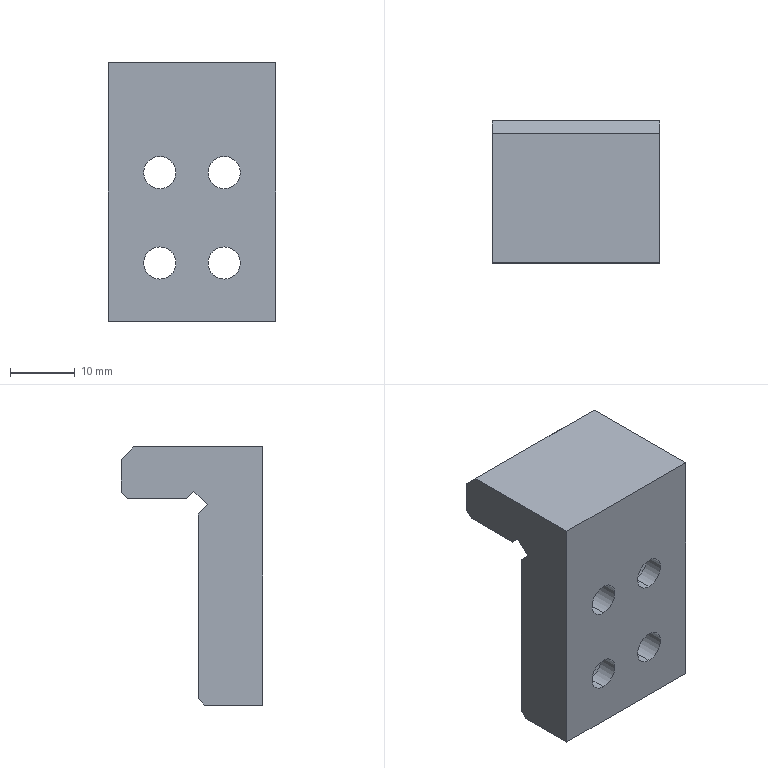Part | SolidWorks | features Chamfer 2, Cut 2, ICE 2, Extrusion 1, HoleWzd 1 | 1 solid | 28 faces | box 26 x 22 x 40 mm | volume 10641 mm3 | plane 16 | cylinder 12 | commonest cylinder face diameters 5 x8 12 x4
STEP:
#1=CARTESIAN_POINT('',(5.,3.,-3.));
#2=VERTEX_POINT('',#1);
#3=CARTESIAN_POINT('',(5.,3.,9.));
#4=VERTEX_POINT('',#3);
#5=CARTESIAN_POINT('',(5.,3.,3.));
#6=DIRECTION('',(0.,1.,0.));
#7=DIRECTION('',(0.,0.,1.));
#8=AXIS2_PLACEMENT_3D('',#5,#6,#7);
#9=CIRCLE('',#8,6.);
#10=EDGE_CURVE('',#2,#4,#9,.T.);
#11=ORIENTED_EDGE('',*,*,#10,.F.);
#12=CARTESIAN_POINT('',(5.,10.,-3.));
#13=VERTEX_POINT('',#12);
#14=CARTESIAN_POINT('',(5.,3.,-3.));
#15=DIRECTION('',(0.,1.,0.));
#16=VECTOR('',#15,1000.);
#17=LINE('',#14,#16);
#18=EDGE_CURVE('',#2,#13,#17,.T.);
#19=ORIENTED_EDGE('',*,*,#18,.T.);
#20=CARTESIAN_POINT('',(5.,10.,9.));
#21=VERTEX_POINT('',#20);
#22=CARTESIAN_POINT('',(5.,10.,3.));
#23=DIRECTION('',(0.,1.,0.));
#24=DIRECTION('',(0.,0.,1.));
#25=AXIS2_PLACEMENT_3D('',#22,#23,#24);
#26=CIRCLE('',#25,6.);
#27=EDGE_CURVE('',#13,#21,#26,.T.);
#28=ORIENTED_EDGE('',*,*,#27,.T.);
#29=CARTESIAN_POINT('',(5.,3.,9.));
#30=DIRECTION('',(0.,1.,0.));
#31=VECTOR('',#30,1000.);
#32=LINE('',#29,#31);
#33=EDGE_CURVE('',#4,#21,#32,.T.);
#34=ORIENTED_EDGE('',*,*,#33,.F.);
#35=EDGE_LOOP('',(#11,#19,#28,#34));
#36=FACE_OUTER_BOUND('',#35,.T.);
#37=CARTESIAN_POINT('',(5.,3.,3.));
#38=DIRECTION('',(0.,1.,0.));
#39=DIRECTION('',(0.,0.,1.));
#40=AXIS2_PLACEMENT_3D('',#37,#38,#39);
#41=CYLINDRICAL_SURFACE('',#40,6.);
#42=ADVANCED_FACE('',(#36),#41,.F.);
#43=CARTESIAN_POINT('',(-5.,3.,-17.));
#44=VERTEX_POINT('',#43);
#45=CARTESIAN_POINT('',(-5.,3.,-5.));
#46=VERTEX_POINT('',#45);
#47=CARTESIAN_POINT('',(-5.,3.,-11.));
#48=DIRECTION('',(0.,1.,0.));
#49=DIRECTION('',(0.,0.,1.));
#50=AXIS2_PLACEMENT_3D('',#47,#48,#49);
#51=CIRCLE('',#50,6.);
#52=EDGE_CURVE('',#44,#46,#51,.T.);
#53=ORIENTED_EDGE('',*,*,#52,.F.);
#54=CARTESIAN_POINT('',(-5.,10.,-17.));
#55=VERTEX_POINT('',#54);
#56=CARTESIAN_POINT('',(-5.,3.,-17.));
#57=DIRECTION('',(0.,1.,0.));
#58=VECTOR('',#57,1000.);
#59=LINE('',#56,#58);
#60=EDGE_CURVE('',#44,#55,#59,.T.);
#61=ORIENTED_EDGE('',*,*,#60,.T.);
#62=CARTESIAN_POINT('',(-5.,10.,-5.));
#63=VERTEX_POINT('',#62);
#64=CARTESIAN_POINT('',(-5.,10.,-11.));
#65=DIRECTION('',(0.,1.,0.));
#66=DIRECTION('',(0.,0.,1.));
#67=AXIS2_PLACEMENT_3D('',#64,#65,#66);
#68=CIRCLE('',#67,6.);
#69=EDGE_CURVE('',#55,#63,#68,.T.);
#70=ORIENTED_EDGE('',*,*,#69,.T.);
#71=CARTESIAN_POINT('',(-5.,3.,-5.));
#72=DIRECTION('',(0.,1.,0.));
#73=VECTOR('',#72,1000.);
#74=LINE('',#71,#73);
#75=EDGE_CURVE('',#46,#63,#74,.T.);
#76=ORIENTED_EDGE('',*,*,#75,.F.);
#77=EDGE_LOOP('',(#53,#61,#70,#76));
#78=FACE_OUTER_BOUND('',#77,.T.);
#79=CARTESIAN_POINT('',(-5.,3.,-11.));
#80=DIRECTION('',(0.,1.,0.));
#81=DIRECTION('',(0.,0.,1.));
#82=AXIS2_PLACEMENT_3D('',#79,#80,#81);
#83=CYLINDRICAL_SURFACE('',#82,6.);
#84=ADVANCED_FACE('',(#78),#83,.F.);
#85=CARTESIAN_POINT('',(5.,0.,-13.5));
#86=VERTEX_POINT('',#85);
#87=CARTESIAN_POINT('',(5.,0.,-8.5));
#88=VERTEX_POINT('',#87);
#89=CARTESIAN_POINT('',(5.,0.,-11.));
#90=DIRECTION('',(0.,1.,0.));
#91=DIRECTION('',(0.,0.,1.));
#92=AXIS2_PLACEMENT_3D('',#89,#90,#91);
#93=CIRCLE('',#92,2.5);
#94=EDGE_CURVE('',#86,#88,#93,.T.);
#95=ORIENTED_EDGE('',*,*,#94,.F.);
#96=CARTESIAN_POINT('',(5.,10.,-13.5));
#97=VERTEX_POINT('',#96);
#98=CARTESIAN_POINT('',(5.,0.,-13.5));
#99=DIRECTION('',(0.,1.,0.));
#100=VECTOR('',#99,1000.);
#101=LINE('',#98,#100);
#102=EDGE_CURVE('',#86,#97,#101,.T.);
#103=ORIENTED_EDGE('',*,*,#102,.T.);
#104=CARTESIAN_POINT('',(5.,10.,-8.5));
#105=VERTEX_POINT('',#104);
#106=CARTESIAN_POINT('',(5.,10.,-11.));
#107=DIRECTION('',(0.,1.,0.));
#108=DIRECTION('',(0.,0.,1.));
#109=AXIS2_PLACEMENT_3D('',#106,#107,#108);
#110=CIRCLE('',#109,2.5);
#111=EDGE_CURVE('',#97,#105,#110,.T.);
#112=ORIENTED_EDGE('',*,*,#111,.T.);
#113=CARTESIAN_POINT('',(5.,0.,-8.5));
#114=DIRECTION('',(0.,1.,0.));
#115=VECTOR('',#114,1000.);
#116=LINE('',#113,#115);
#117=EDGE_CURVE('',#88,#105,#116,.T.);
#118=ORIENTED_EDGE('',*,*,#117,.F.);
#119=EDGE_LOOP('',(#95,#103,#112,#118));
#120=FACE_OUTER_BOUND('',#119,.T.);
#121=CARTESIAN_POINT('',(5.,0.,-11.));
#122=DIRECTION('',(0.,1.,0.));
#123=DIRECTION('',(0.,0.,1.));
#124=AXIS2_PLACEMENT_3D('',#121,#122,#123);
#125=CYLINDRICAL_SURFACE('',#124,2.5);
#126=ADVANCED_FACE('',(#120),#125,.F.);
#127=CARTESIAN_POINT('',(-5.,0.,0.5));
#128=VERTEX_POINT('',#127);
#129=CARTESIAN_POINT('',(-5.,0.,5.5));
#130=VERTEX_POINT('',#129);
#131=CARTESIAN_POINT('',(-5.,0.,3.));
#132=DIRECTION('',(0.,1.,0.));
#133=DIRECTION('',(0.,0.,1.));
#134=AXIS2_PLACEMENT_3D('',#131,#132,#133);
#135=CIRCLE('',#134,2.5);
#136=EDGE_CURVE('',#128,#130,#135,.T.);
#137=ORIENTED_EDGE('',*,*,#136,.F.);
#138=CARTESIAN_POINT('',(-5.,10.,0.5));
#139=VERTEX_POINT('',#138);
#140=CARTESIAN_POINT('',(-5.,0.,0.5));
#141=DIRECTION('',(0.,1.,0.));
#142=VECTOR('',#141,1000.);
#143=LINE('',#140,#142);
#144=EDGE_CURVE('',#128,#139,#143,.T.);
#145=ORIENTED_EDGE('',*,*,#144,.T.);
#146=CARTESIAN_POINT('',(-5.,10.,5.5));
#147=VERTEX_POINT('',#146);
#148=CARTESIAN_POINT('',(-5.,10.,3.));
#149=DIRECTION('',(0.,1.,0.));
#150=DIRECTION('',(0.,0.,1.));
#151=AXIS2_PLACEMENT_3D('',#148,#149,#150);
#152=CIRCLE('',#151,2.5);
#153=EDGE_CURVE('',#139,#147,#152,.T.);
#154=ORIENTED_EDGE('',*,*,#153,.T.);
#155=CARTESIAN_POINT('',(-5.,0.,5.5));
#156=DIRECTION('',(0.,1.,0.));
#157=VECTOR('',#156,1000.);
#158=LINE('',#155,#157);
#159=EDGE_CURVE('',#130,#147,#158,.T.);
#160=ORIENTED_EDGE('',*,*,#159,.F.);
#161=EDGE_LOOP('',(#137,#145,#154,#160));
#162=FACE_OUTER_BOUND('',#161,.T.);
#163=CARTESIAN_POINT('',(-5.,0.,3.));
#164=DIRECTION('',(0.,1.,0.));
#165=DIRECTION('',(0.,0.,1.));
#166=AXIS2_PLACEMENT_3D('',#163,#164,#165);
#167=CYLINDRICAL_SURFACE('',#166,2.5);
#168=ADVANCED_FACE('',(#162),#167,.F.);
#169=CARTESIAN_POINT('',(-5.,0.,-13.5));
#170=VERTEX_POINT('',#169);
#171=CARTESIAN_POINT('',(-5.,0.,-8.5));
#172=VERTEX_POINT('',#171);
#173=CARTESIAN_POINT('',(-5.,0.,-11.));
#174=DIRECTION('',(0.,1.,0.));
#175=DIRECTION('',(0.,0.,1.));
#176=AXIS2_PLACEMENT_3D('',#173,#174,#175);
#177=CIRCLE('',#176,2.5);
#178=EDGE_CURVE('',#170,#172,#177,.T.);
#179=ORIENTED_EDGE('',*,*,#178,.F.);
#180=CARTESIAN_POINT('',(-5.,3.,-13.5));
#181=VERTEX_POINT('',#180);
#182=CARTESIAN_POINT('',(-5.,10.,-13.5));
#183=DIRECTION('',(0.,1.,0.));
#184=VECTOR('',#183,1000.);
#185=LINE('',#182,#184);
#186=EDGE_CURVE('',#170,#181,#185,.T.);
#187=ORIENTED_EDGE('',*,*,#186,.T.);
#188=CARTESIAN_POINT('',(-5.,3.,-8.5));
#189=VERTEX_POINT('',#188);
#190=CARTESIAN_POINT('',(-5.,3.,-11.));
#191=DIRECTION('',(0.,-1.,0.));
#192=DIRECTION('',(0.,0.,1.));
#193=AXIS2_PLACEMENT_3D('',#190,#191,#192);
#194=CIRCLE('',#193,2.5);
#195=EDGE_CURVE('',#189,#181,#194,.T.);
#196=ORIENTED_EDGE('',*,*,#195,.F.);
#197=CARTESIAN_POINT('',(-5.,10.,-8.5));
#198=DIRECTION('',(0.,1.,0.));
#199=VECTOR('',#198,1000.);
#200=LINE('',#197,#199);
#201=EDGE_CURVE('',#172,#189,#200,.T.);
#202=ORIENTED_EDGE('',*,*,#201,.F.);
#203=EDGE_LOOP('',(#179,#187,#196,#202));
#204=FACE_OUTER_BOUND('',#203,.T.);
#205=CARTESIAN_POINT('',(-5.,10.,-11.));
#206=DIRECTION('',(0.,1.,0.));
#207=DIRECTION('',(0.,0.,1.));
#208=AXIS2_PLACEMENT_3D('',#205,#206,#207);
#209=CYLINDRICAL_SURFACE('',#208,2.5);
#210=ADVANCED_FACE('',(#204),#209,.F.);
#211=CARTESIAN_POINT('',(5.,0.,0.5));
#212=VERTEX_POINT('',#211);
#213=CARTESIAN_POINT('',(5.,0.,5.5));
#214=VERTEX_POINT('',#213);
#215=CARTESIAN_POINT('',(5.,0.,3.));
#216=DIRECTION('',(0.,1.,0.));
#217=DIRECTION('',(0.,0.,1.));
#218=AXIS2_PLACEMENT_3D('',#215,#216,#217);
#219=CIRCLE('',#218,2.5);
#220=EDGE_CURVE('',#212,#214,#219,.T.);
#221=ORIENTED_EDGE('',*,*,#220,.F.);
#222=CARTESIAN_POINT('',(5.,3.,0.5));
#223=VERTEX_POINT('',#222);
#224=CARTESIAN_POINT('',(5.,10.,0.5));
#225=DIRECTION('',(0.,1.,0.));
#226=VECTOR('',#225,1000.);
#227=LINE('',#224,#226);
#228=EDGE_CURVE('',#212,#223,#227,.T.);
#229=ORIENTED_EDGE('',*,*,#228,.T.);
#230=CARTESIAN_POINT('',(5.,3.,5.5));
#231=VERTEX_POINT('',#230);
#232=CARTESIAN_POINT('',(5.,3.,3.));
#233=DIRECTION('',(0.,-1.,0.));
#234=DIRECTION('',(0.,0.,1.));
#235=AXIS2_PLACEMENT_3D('',#232,#233,#234);
#236=CIRCLE('',#235,2.5);
#237=EDGE_CURVE('',#231,#223,#236,.T.);
#238=ORIENTED_EDGE('',*,*,#237,.F.);
#239=CARTESIAN_POINT('',(5.,10.,5.5));
#240=DIRECTION('',(0.,1.,0.));
#241=VECTOR('',#240,1000.);
#242=LINE('',#239,#241);
#243=EDGE_CURVE('',#214,#231,#242,.T.);
#244=ORIENTED_EDGE('',*,*,#243,.F.);
#245=EDGE_LOOP('',(#221,#229,#238,#244));
#246=FACE_OUTER_BOUND('',#245,.T.);
#247=CARTESIAN_POINT('',(5.,10.,3.));
#248=DIRECTION('',(0.,1.,0.));
#249=DIRECTION('',(0.,0.,1.));
#250=AXIS2_PLACEMENT_3D('',#247,#248,#249);
#251=CYLINDRICAL_SURFACE('',#250,2.5);
#252=ADVANCED_FACE('',(#246),#251,.F.);
#253=ORIENTED_EDGE('',*,*,#228,.F.);
#254=CARTESIAN_POINT('',(5.,0.,3.));
#255=DIRECTION('',(0.,1.,0.));
#256=DIRECTION('',(0.,0.,1.));
#257=AXIS2_PLACEMENT_3D('',#254,#255,#256);
#258=CIRCLE('',#257,2.5);
#259=EDGE_CURVE('',#214,#212,#258,.T.);
#260=ORIENTED_EDGE('',*,*,#259,.F.);
#261=ORIENTED_EDGE('',*,*,#243,.T.);
#262=CARTESIAN_POINT('',(5.,3.,3.));
#263=DIRECTION('',(0.,-1.,0.));
#264=DIRECTION('',(0.,0.,1.));
#265=AXIS2_PLACEMENT_3D('',#262,#263,#264);
#266=CIRCLE('',#265,2.5);
#267=EDGE_CURVE('',#223,#231,#266,.T.);
#268=ORIENTED_EDGE('',*,*,#267,.F.);
#269=EDGE_LOOP('',(#253,#260,#261,#268));
#270=FACE_OUTER_BOUND('',#269,.T.);
#271=CARTESIAN_POINT('',(5.,10.,3.));
#272=DIRECTION('',(0.,1.,0.));
#273=DIRECTION('',(0.,0.,1.));
#274=AXIS2_PLACEMENT_3D('',#271,#272,#273);
#275=CYLINDRICAL_SURFACE('',#274,2.5);
#276=ADVANCED_FACE('',(#270),#275,.F.);
#277=ORIENTED_EDGE('',*,*,#186,.F.);
#278=CARTESIAN_POINT('',(-5.,0.,-11.));
#279=DIRECTION('',(0.,1.,0.));
#280=DIRECTION('',(0.,0.,1.));
#281=AXIS2_PLACEMENT_3D('',#278,#279,#280);
#282=CIRCLE('',#281,2.5);
#283=EDGE_CURVE('',#172,#170,#282,.T.);
#284=ORIENTED_EDGE('',*,*,#283,.F.);
#285=ORIENTED_EDGE('',*,*,#201,.T.);
#286=CARTESIAN_POINT('',(-5.,3.,-11.));
#287=DIRECTION('',(0.,-1.,0.));
#288=DIRECTION('',(0.,0.,1.));
#289=AXIS2_PLACEMENT_3D('',#286,#287,#288);
#290=CIRCLE('',#289,2.5);
#291=EDGE_CURVE('',#181,#189,#290,.T.);
#292=ORIENTED_EDGE('',*,*,#291,.F.);
#293=EDGE_LOOP('',(#277,#284,#285,#292));
#294=FACE_OUTER_BOUND('',#293,.T.);
#295=CARTESIAN_POINT('',(-5.,10.,-11.));
#296=DIRECTION('',(0.,1.,0.));
#297=DIRECTION('',(0.,0.,1.));
#298=AXIS2_PLACEMENT_3D('',#295,#296,#297);
#299=CYLINDRICAL_SURFACE('',#298,2.5);
#300=ADVANCED_FACE('',(#294),#299,.F.);
#301=CARTESIAN_POINT('',(13.,9.,-20.));
#302=VERTEX_POINT('',#301);
#303=CARTESIAN_POINT('',(13.,0.,-20.));
#304=VERTEX_POINT('',#303);
#305=CARTESIAN_POINT('',(13.,10.,-20.));
#306=DIRECTION('',(0.,-1.,0.));
#307=VECTOR('',#306,1000.);
#308=LINE('',#305,#307);
#309=EDGE_CURVE('',#302,#304,#308,.T.);
#310=ORIENTED_EDGE('',*,*,#309,.F.);
#311=CARTESIAN_POINT('',(13.,10.,-19.));
#312=VERTEX_POINT('',#311);
#313=CARTESIAN_POINT('',(13.,10.,-19.));
#314=DIRECTION('',(0.,0.7071,0.7071));
#315=VECTOR('',#314,1000.);
#316=LINE('',#313,#315);
#317=EDGE_CURVE('',#302,#312,#316,.T.);
#318=ORIENTED_EDGE('',*,*,#317,.T.);
#319=CARTESIAN_POINT('',(13.,10.,9.607));
#320=VERTEX_POINT('',#319);
#321=CARTESIAN_POINT('',(13.,10.,-20.));
#322=DIRECTION('',(0.,0.,-1.));
#323=VECTOR('',#322,1000.);
#324=LINE('',#321,#323);
#325=EDGE_CURVE('',#320,#312,#324,.T.);
#326=ORIENTED_EDGE('',*,*,#325,.F.);
#327=CARTESIAN_POINT('',(13.,8.59,11.025));
#328=VERTEX_POINT('',#327);
#329=CARTESIAN_POINT('',(13.,10.963,8.638));
#330=DIRECTION('',(0.,0.705,-0.7092));
#331=VECTOR('',#330,1000.);
#332=LINE('',#329,#331);
#333=EDGE_CURVE('',#328,#320,#332,.T.);
#334=ORIENTED_EDGE('',*,*,#333,.F.);
#335=CARTESIAN_POINT('',(13.,10.718,13.14));
#336=VERTEX_POINT('',#335);
#337=CARTESIAN_POINT('',(13.,10.718,13.14));
#338=DIRECTION('',(0.,-0.7092,-0.705));
#339=VECTOR('',#338,1000.);
#340=LINE('',#337,#339);
#341=EDGE_CURVE('',#336,#328,#340,.T.);
#342=ORIENTED_EDGE('',*,*,#341,.F.);
#343=CARTESIAN_POINT('',(13.,11.851,12.));
#344=VERTEX_POINT('',#343);
#345=CARTESIAN_POINT('',(13.,13.091,10.753));
#346=DIRECTION('',(0.,-0.705,0.7092));
#347=VECTOR('',#346,1000.);
#348=LINE('',#345,#347);
#349=EDGE_CURVE('',#344,#336,#348,.T.);
#350=ORIENTED_EDGE('',*,*,#349,.F.);
#351=CARTESIAN_POINT('',(13.,21.,12.));
#352=VERTEX_POINT('',#351);
#353=CARTESIAN_POINT('',(13.,22.,12.));
#354=DIRECTION('',(0.,-1.,0.));
#355=VECTOR('',#354,1000.);
#356=LINE('',#353,#355);
#357=EDGE_CURVE('',#352,#344,#356,.T.);
#358=ORIENTED_EDGE('',*,*,#357,.F.);
#359=CARTESIAN_POINT('',(13.,22.,13.));
#360=VERTEX_POINT('',#359);
#361=CARTESIAN_POINT('',(13.,22.,13.));
#362=DIRECTION('',(0.,0.7071,0.7071));
#363=VECTOR('',#362,1000.);
#364=LINE('',#361,#363);
#365=EDGE_CURVE('',#352,#360,#364,.T.);
#366=ORIENTED_EDGE('',*,*,#365,.T.);
#367=CARTESIAN_POINT('',(13.,22.,18.));
#368=VERTEX_POINT('',#367);
#369=CARTESIAN_POINT('',(13.,22.,20.));
#370=DIRECTION('',(0.,0.,-1.));
#371=VECTOR('',#370,1000.);
#372=LINE('',#369,#371);
#373=EDGE_CURVE('',#368,#360,#372,.T.);
#374=ORIENTED_EDGE('',*,*,#373,.F.);
#375=CARTESIAN_POINT('',(13.,20.,20.));
#376=VERTEX_POINT('',#375);
#377=CARTESIAN_POINT('',(13.,22.,18.));
#378=DIRECTION('',(0.,-0.7071,0.7071));
#379=VECTOR('',#378,1000.);
#380=LINE('',#377,#379);
#381=EDGE_CURVE('',#368,#376,#380,.T.);
#382=ORIENTED_EDGE('',*,*,#381,.T.);
#383=CARTESIAN_POINT('',(13.,0.,20.));
#384=VERTEX_POINT('',#383);
#385=CARTESIAN_POINT('',(13.,10.,20.));
#386=DIRECTION('',(0.,-1.,0.));
#387=VECTOR('',#386,1000.);
#388=LINE('',#385,#387);
#389=EDGE_CURVE('',#376,#384,#388,.T.);
#390=ORIENTED_EDGE('',*,*,#389,.T.);
#391=CARTESIAN_POINT('',(13.,0.,-20.));
#392=DIRECTION('',(0.,0.,-1.));
#393=VECTOR('',#392,1000.);
#394=LINE('',#391,#393);
#395=EDGE_CURVE('',#384,#304,#394,.T.);
#396=ORIENTED_EDGE('',*,*,#395,.T.);
#397=EDGE_LOOP('',(#310,#318,#326,#334,#342,#350,#358,#366,#374,#382,#390,#396));
#398=FACE_OUTER_BOUND('',#397,.T.);
#399=CARTESIAN_POINT('',(13.,10.,-20.));
#400=DIRECTION('',(-1.,0.,0.));
#401=DIRECTION('',(0.,0.,1.));
#402=AXIS2_PLACEMENT_3D('',#399,#400,#401);
#403=PLANE('',#402);
#404=ADVANCED_FACE('',(#398),#403,.F.);
#405=CARTESIAN_POINT('',(-13.,9.,-20.));
#406=VERTEX_POINT('',#405);
#407=CARTESIAN_POINT('',(-13.,0.,-20.));
#408=VERTEX_POINT('',#407);
#409=CARTESIAN_POINT('',(-13.,10.,-20.));
#410=DIRECTION('',(0.,-1.,0.));
#411=VECTOR('',#410,1000.);
#412=LINE('',#409,#411);
#413=EDGE_CURVE('',#406,#408,#412,.T.);
#414=ORIENTED_EDGE('',*,*,#413,.F.);
#415=CARTESIAN_POINT('',(13.,9.,-20.));
#416=DIRECTION('',(1.,0.,0.));
#417=VECTOR('',#416,1000.);
#418=LINE('',#415,#417);
#419=EDGE_CURVE('',#406,#302,#418,.T.);
#420=ORIENTED_EDGE('',*,*,#419,.T.);
#421=ORIENTED_EDGE('',*,*,#309,.T.);
#422=CARTESIAN_POINT('',(-13.,0.,-20.));
#423=DIRECTION('',(-1.,0.,0.));
#424=VECTOR('',#423,1000.);
#425=LINE('',#422,#424);
#426=EDGE_CURVE('',#304,#408,#425,.T.);
#427=ORIENTED_EDGE('',*,*,#426,.T.);
#428=EDGE_LOOP('',(#414,#420,#421,#427));
#429=FACE_OUTER_BOUND('',#428,.T.);
#430=CARTESIAN_POINT('',(-13.,10.,-20.));
#431=DIRECTION('',(0.,0.,1.));
#432=DIRECTION('',(1.,0.,0.));
#433=AXIS2_PLACEMENT_3D('',#430,#431,#432);
#434=PLANE('',#433);
#435=ADVANCED_FACE('',(#429),#434,.F.);
#436=CARTESIAN_POINT('',(-13.,10.,-19.));
#437=VERTEX_POINT('',#436);
#438=CARTESIAN_POINT('',(-13.,10.,9.607));
#439=VERTEX_POINT('',#438);
#440=CARTESIAN_POINT('',(-13.,10.,-20.));
#441=DIRECTION('',(0.,0.,1.));
#442=VECTOR('',#441,1000.);
#443=LINE('',#440,#442);
#444=EDGE_CURVE('',#437,#439,#443,.T.);
#445=ORIENTED_EDGE('',*,*,#444,.F.);
#446=CARTESIAN_POINT('',(-13.,10.,-19.));
#447=DIRECTION('',(0.,-0.7071,-0.7071));
#448=VECTOR('',#447,1000.);
#449=LINE('',#446,#448);
#450=EDGE_CURVE('',#437,#406,#449,.T.);
#451=ORIENTED_EDGE('',*,*,#450,.T.);
#452=ORIENTED_EDGE('',*,*,#413,.T.);
#453=CARTESIAN_POINT('',(-13.,0.,20.));
#454=VERTEX_POINT('',#453);
#455=CARTESIAN_POINT('',(-13.,0.,-20.));
#456=DIRECTION('',(0.,0.,1.));
#457=VECTOR('',#456,1000.);
#458=LINE('',#455,#457);
#459=EDGE_CURVE('',#408,#454,#458,.T.);
#460=ORIENTED_EDGE('',*,*,#459,.T.);
#461=CARTESIAN_POINT('',(-13.,20.,20.));
#462=VERTEX_POINT('',#461);
#463=CARTESIAN_POINT('',(-13.,10.,20.));
#464=DIRECTION('',(0.,-1.,0.));
#465=VECTOR('',#464,1000.);
#466=LINE('',#463,#465);
#467=EDGE_CURVE('',#462,#454,#466,.T.);
#468=ORIENTED_EDGE('',*,*,#467,.F.);
#469=CARTESIAN_POINT('',(-13.,22.,18.));
#470=VERTEX_POINT('',#469);
#471=CARTESIAN_POINT('',(-13.,22.,18.));
#472=DIRECTION('',(0.,0.7071,-0.7071));
#473=VECTOR('',#472,1000.);
#474=LINE('',#471,#473);
#475=EDGE_CURVE('',#462,#470,#474,.T.);
#476=ORIENTED_EDGE('',*,*,#475,.T.);
#477=CARTESIAN_POINT('',(-13.,22.,13.));
#478=VERTEX_POINT('',#477);
#479=CARTESIAN_POINT('',(-13.,22.,20.));
#480=DIRECTION('',(0.,0.,1.));
#481=VECTOR('',#480,1000.);
#482=LINE('',#479,#481);
#483=EDGE_CURVE('',#478,#470,#482,.T.);
#484=ORIENTED_EDGE('',*,*,#483,.F.);
#485=CARTESIAN_POINT('',(-13.,21.,12.));
#486=VERTEX_POINT('',#485);
#487=CARTESIAN_POINT('',(-13.,22.,13.));
#488=DIRECTION('',(0.,-0.7071,-0.7071));
#489=VECTOR('',#488,1000.);
#490=LINE('',#487,#489);
#491=EDGE_CURVE('',#478,#486,#490,.T.);
#492=ORIENTED_EDGE('',*,*,#491,.T.);
#493=CARTESIAN_POINT('',(-13.,11.851,12.));
#494=VERTEX_POINT('',#493);
#495=CARTESIAN_POINT('',(-13.,22.,12.));
#496=DIRECTION('',(0.,-1.,0.));
#497=VECTOR('',#496,1000.);
#498=LINE('',#495,#497);
#499=EDGE_CURVE('',#486,#494,#498,.T.);
#500=ORIENTED_EDGE('',*,*,#499,.T.);
#501=CARTESIAN_POINT('',(-13.,10.718,13.14));
#502=VERTEX_POINT('',#501);
#503=CARTESIAN_POINT('',(-13.,26.931,-3.17));
#504=DIRECTION('',(0.,-0.705,0.7092));
#505=VECTOR('',#504,1000.);
#506=LINE('',#503,#505);
#507=EDGE_CURVE('',#494,#502,#506,.T.);
#508=ORIENTED_EDGE('',*,*,#507,.T.);
#509=CARTESIAN_POINT('',(-13.,8.59,11.025));
#510=VERTEX_POINT('',#509);
#511=CARTESIAN_POINT('',(-13.,-6.213,-3.69));
#512=DIRECTION('',(0.,-0.7092,-0.705));
#513=VECTOR('',#512,1000.);
#514=LINE('',#511,#513);
#515=EDGE_CURVE('',#502,#510,#514,.T.);
#516=ORIENTED_EDGE('',*,*,#515,.T.);
#517=CARTESIAN_POINT('',(-13.,24.803,-5.285));
#518=DIRECTION('',(0.,0.705,-0.7092));
#519=VECTOR('',#518,1000.);
#520=LINE('',#517,#519);
#521=EDGE_CURVE('',#510,#439,#520,.T.);
#522=ORIENTED_EDGE('',*,*,#521,.T.);
#523=EDGE_LOOP('',(#445,#451,#452,#460,#468,#476,#484,#492,#500,#508,#516,#522));
#524=FACE_OUTER_BOUND('',#523,.T.);
#525=CARTESIAN_POINT('',(-13.,10.,-20.));
#526=DIRECTION('',(1.,0.,0.));
#527=DIRECTION('',(0.,0.,-1.));
#528=AXIS2_PLACEMENT_3D('',#525,#526,#527);
#529=PLANE('',#528);
#530=ADVANCED_FACE('',(#524),#529,.F.);
#531=ORIENTED_EDGE('',*,*,#389,.F.);
#532=CARTESIAN_POINT('',(-13.,20.,20.));
#533=DIRECTION('',(-1.,0.,0.));
#534=VECTOR('',#533,1000.);
#535=LINE('',#532,#534);
#536=EDGE_CURVE('',#376,#462,#535,.T.);
#537=ORIENTED_EDGE('',*,*,#536,.T.);
#538=ORIENTED_EDGE('',*,*,#467,.T.);
#539=CARTESIAN_POINT('',(-13.,0.,20.));
#540=DIRECTION('',(1.,0.,0.));
#541=VECTOR('',#540,1000.);
#542=LINE('',#539,#541);
#543=EDGE_CURVE('',#454,#384,#542,.T.);
#544=ORIENTED_EDGE('',*,*,#543,.T.);
#545=EDGE_LOOP('',(#531,#537,#538,#544));
#546=FACE_OUTER_BOUND('',#545,.T.);
#547=CARTESIAN_POINT('',(-13.,10.,20.));
#548=DIRECTION('',(0.,0.,-1.));
#549=DIRECTION('',(-1.,0.,0.));
#550=AXIS2_PLACEMENT_3D('',#547,#548,#549);
#551=PLANE('',#550);
#552=ADVANCED_FACE('',(#546),#551,.F.);
#553=CARTESIAN_POINT('',(-5.,10.,-11.));
#554=DIRECTION('',(0.,1.,0.));
#555=DIRECTION('',(0.,0.,1.));
#556=AXIS2_PLACEMENT_3D('',#553,#554,#555);
#557=CIRCLE('',#556,6.);
#558=EDGE_CURVE('',#63,#55,#557,.T.);
#559=ORIENTED_EDGE('',*,*,#558,.F.);
#560=ORIENTED_EDGE('',*,*,#69,.F.);
#561=EDGE_LOOP('',(#559,#560));
#562=FACE_BOUND('',#561,.T.);
#563=CARTESIAN_POINT('',(5.,10.,3.));
#564=DIRECTION('',(0.,1.,0.));
#565=DIRECTION('',(0.,0.,1.));
#566=AXIS2_PLACEMENT_3D('',#563,#564,#565);
#567=CIRCLE('',#566,6.);
#568=EDGE_CURVE('',#21,#13,#567,.T.);
#569=ORIENTED_EDGE('',*,*,#568,.F.);
#570=ORIENTED_EDGE('',*,*,#27,.F.);
#571=EDGE_LOOP('',(#569,#570));
#572=FACE_BOUND('',#571,.T.);
#573=CARTESIAN_POINT('',(5.,10.,-11.));
#574=DIRECTION('',(0.,1.,0.));
#575=DIRECTION('',(0.,0.,1.));
#576=AXIS2_PLACEMENT_3D('',#573,#574,#575);
#577=CIRCLE('',#576,2.5);
#578=EDGE_CURVE('',#105,#97,#577,.T.);
#579=ORIENTED_EDGE('',*,*,#578,.F.);
#580=ORIENTED_EDGE('',*,*,#111,.F.);
#581=EDGE_LOOP('',(#579,#580));
#582=FACE_BOUND('',#581,.T.);
#583=CARTESIAN_POINT('',(-5.,10.,3.));
#584=DIRECTION('',(0.,1.,0.));
#585=DIRECTION('',(0.,0.,1.));
#586=AXIS2_PLACEMENT_3D('',#583,#584,#585);
#587=CIRCLE('',#586,2.5);
#588=EDGE_CURVE('',#147,#139,#587,.T.);
#589=ORIENTED_EDGE('',*,*,#588,.F.);
#590=ORIENTED_EDGE('',*,*,#153,.F.);
#591=EDGE_LOOP('',(#589,#590));
#592=FACE_BOUND('',#591,.T.);
#593=ORIENTED_EDGE('',*,*,#325,.T.);
#594=CARTESIAN_POINT('',(-13.,10.,-19.));
#595=DIRECTION('',(-1.,0.,0.));
#596=VECTOR('',#595,1000.);
#597=LINE('',#594,#596);
#598=EDGE_CURVE('',#312,#437,#597,.T.);
#599=ORIENTED_EDGE('',*,*,#598,.T.);
#600=ORIENTED_EDGE('',*,*,#444,.T.);
#601=CARTESIAN_POINT('',(0.,10.,9.607));
#602=DIRECTION('',(-1.,0.,0.));
#603=VECTOR('',#602,1000.);
#604=LINE('',#601,#603);
#605=EDGE_CURVE('',#320,#439,#604,.T.);
#606=ORIENTED_EDGE('',*,*,#605,.F.);
#607=EDGE_LOOP('',(#593,#599,#600,#606));
#608=FACE_OUTER_BOUND('',#607,.T.);
#609=CARTESIAN_POINT('',(0.,10.,0.));
#610=DIRECTION('',(0.,1.,0.));
#611=DIRECTION('',(0.,0.,1.));
#612=AXIS2_PLACEMENT_3D('',#609,#610,#611);
#613=PLANE('',#612);
#614=ADVANCED_FACE('',(#562,#572,#582,#592,#608),#613,.T.);
#615=CARTESIAN_POINT('',(5.,0.,-11.));
#616=DIRECTION('',(0.,1.,0.));
#617=DIRECTION('',(0.,0.,1.));
#618=AXIS2_PLACEMENT_3D('',#615,#616,#617);
#619=CIRCLE('',#618,2.5);
#620=EDGE_CURVE('',#88,#86,#619,.T.);
#621=ORIENTED_EDGE('',*,*,#620,.T.);
#622=ORIENTED_EDGE('',*,*,#94,.T.);
#623=EDGE_LOOP('',(#621,#622));
#624=FACE_BOUND('',#623,.T.);
#625=CARTESIAN_POINT('',(-5.,0.,3.));
#626=DIRECTION('',(0.,1.,0.));
#627=DIRECTION('',(0.,0.,1.));
#628=AXIS2_PLACEMENT_3D('',#625,#626,#627);
#629=CIRCLE('',#628,2.5);
#630=EDGE_CURVE('',#130,#128,#629,.T.);
#631=ORIENTED_EDGE('',*,*,#630,.T.);
#632=ORIENTED_EDGE('',*,*,#136,.T.);
#633=EDGE_LOOP('',(#631,#632));
#634=FACE_BOUND('',#633,.T.);
#635=ORIENTED_EDGE('',*,*,#283,.T.);
#636=ORIENTED_EDGE('',*,*,#178,.T.);
#637=EDGE_LOOP('',(#635,#636));
#638=FACE_BOUND('',#637,.T.);
#639=ORIENTED_EDGE('',*,*,#259,.T.);
#640=ORIENTED_EDGE('',*,*,#220,.T.);
#641=EDGE_LOOP('',(#639,#640));
#642=FACE_BOUND('',#641,.T.);
#643=ORIENTED_EDGE('',*,*,#395,.F.);
#644=ORIENTED_EDGE('',*,*,#543,.F.);
#645=ORIENTED_EDGE('',*,*,#459,.F.);
#646=ORIENTED_EDGE('',*,*,#426,.F.);
#647=EDGE_LOOP('',(#643,#644,#645,#646));
#648=FACE_OUTER_BOUND('',#647,.T.);
#649=CARTESIAN_POINT('',(0.,0.,0.));
#650=DIRECTION('',(0.,1.,0.));
#651=DIRECTION('',(0.,0.,1.));
#652=AXIS2_PLACEMENT_3D('',#649,#650,#651);
#653=PLANE('',#652);
#654=ADVANCED_FACE('',(#624,#634,#638,#642,#648),#653,.F.);
#655=ORIENTED_EDGE('',*,*,#499,.F.);
#656=CARTESIAN_POINT('',(-13.,21.,12.));
#657=DIRECTION('',(1.,0.,0.));
#658=VECTOR('',#657,1000.);
#659=LINE('',#656,#658);
#660=EDGE_CURVE('',#486,#352,#659,.T.);
#661=ORIENTED_EDGE('',*,*,#660,.T.);
#662=ORIENTED_EDGE('',*,*,#357,.T.);
#663=CARTESIAN_POINT('',(-13.,11.851,12.));
#664=DIRECTION('',(-1.,0.,0.));
#665=VECTOR('',#664,1000.);
#666=LINE('',#663,#665);
#667=EDGE_CURVE('',#344,#494,#666,.T.);
#668=ORIENTED_EDGE('',*,*,#667,.T.);
#669=EDGE_LOOP('',(#655,#661,#662,#668));
#670=FACE_OUTER_BOUND('',#669,.T.);
#671=CARTESIAN_POINT('',(-13.,22.,12.));
#672=DIRECTION('',(0.,0.,1.));
#673=DIRECTION('',(1.,0.,0.));
#674=AXIS2_PLACEMENT_3D('',#671,#672,#673);
#675=PLANE('',#674);
#676=ADVANCED_FACE('',(#670),#675,.F.);
#677=ORIENTED_EDGE('',*,*,#373,.T.);
#678=CARTESIAN_POINT('',(0.,22.,13.));
#679=DIRECTION('',(-1.,0.,0.));
#680=VECTOR('',#679,1000.);
#681=LINE('',#678,#680);
#682=EDGE_CURVE('',#360,#478,#681,.T.);
#683=ORIENTED_EDGE('',*,*,#682,.T.);
#684=ORIENTED_EDGE('',*,*,#483,.T.);
#685=CARTESIAN_POINT('',(0.,22.,18.));
#686=DIRECTION('',(1.,0.,0.));
#687=VECTOR('',#686,1000.);
#688=LINE('',#685,#687);
#689=EDGE_CURVE('',#470,#368,#688,.T.);
#690=ORIENTED_EDGE('',*,*,#689,.T.);
#691=EDGE_LOOP('',(#677,#683,#684,#690));
#692=FACE_OUTER_BOUND('',#691,.T.);
#693=CARTESIAN_POINT('',(0.,22.,0.));
#694=DIRECTION('',(0.,-1.,0.));
#695=DIRECTION('',(0.,0.,-1.));
#696=AXIS2_PLACEMENT_3D('',#693,#694,#695);
#697=PLANE('',#696);
#698=ADVANCED_FACE('',(#692),#697,.F.);
#699=CARTESIAN_POINT('',(-18.,10.718,13.14));
#700=DIRECTION('',(1.,0.,0.));
#701=VECTOR('',#700,1000.);
#702=LINE('',#699,#701);
#703=EDGE_CURVE('',#502,#336,#702,.T.);
#704=ORIENTED_EDGE('',*,*,#703,.T.);
#705=ORIENTED_EDGE('',*,*,#341,.T.);
#706=CARTESIAN_POINT('',(-18.,8.59,11.025));
#707=DIRECTION('',(1.,0.,0.));
#708=VECTOR('',#707,1000.);
#709=LINE('',#706,#708);
#710=EDGE_CURVE('',#510,#328,#709,.T.);
#711=ORIENTED_EDGE('',*,*,#710,.F.);
#712=ORIENTED_EDGE('',*,*,#515,.F.);
#713=EDGE_LOOP('',(#704,#705,#711,#712));
#714=FACE_OUTER_BOUND('',#713,.T.);
#715=CARTESIAN_POINT('',(-18.,10.718,13.14));
#716=DIRECTION('',(0.,-0.705,0.7092));
#717=DIRECTION('',(0.,-0.7092,-0.705));
#718=AXIS2_PLACEMENT_3D('',#715,#716,#717);
#719=PLANE('',#718);
#720=ADVANCED_FACE('',(#714),#719,.F.);
#721=ORIENTED_EDGE('',*,*,#710,.T.);
#722=ORIENTED_EDGE('',*,*,#333,.T.);
#723=ORIENTED_EDGE('',*,*,#605,.T.);
#724=ORIENTED_EDGE('',*,*,#521,.F.);
#725=EDGE_LOOP('',(#721,#722,#723,#724));
#726=FACE_OUTER_BOUND('',#725,.T.);
#727=CARTESIAN_POINT('',(-18.,10.963,8.638));
#728=DIRECTION('',(0.,-0.7092,-0.705));
#729=DIRECTION('',(0.,0.705,-0.7092));
#730=AXIS2_PLACEMENT_3D('',#727,#728,#729);
#731=PLANE('',#730);
#732=ADVANCED_FACE('',(#726),#731,.F.);
#733=ORIENTED_EDGE('',*,*,#667,.F.);
#734=ORIENTED_EDGE('',*,*,#349,.T.);
#735=ORIENTED_EDGE('',*,*,#703,.F.);
#736=ORIENTED_EDGE('',*,*,#507,.F.);
#737=EDGE_LOOP('',(#733,#734,#735,#736));
#738=FACE_OUTER_BOUND('',#737,.T.);
#739=CARTESIAN_POINT('',(-18.,13.091,10.753));
#740=DIRECTION('',(0.,0.7092,0.705));
#741=DIRECTION('',(0.,-0.705,0.7092));
#742=AXIS2_PLACEMENT_3D('',#739,#740,#741);
#743=PLANE('',#742);
#744=ADVANCED_FACE('',(#738),#743,.F.);
#745=ORIENTED_EDGE('',*,*,#475,.F.);
#746=ORIENTED_EDGE('',*,*,#536,.F.);
#747=ORIENTED_EDGE('',*,*,#381,.F.);
#748=ORIENTED_EDGE('',*,*,#689,.F.);
#749=EDGE_LOOP('',(#745,#746,#747,#748));
#750=FACE_OUTER_BOUND('',#749,.T.);
#751=CARTESIAN_POINT('',(0.,22.,18.));
#752=DIRECTION('',(0.,-0.7071,-0.7071));
#753=DIRECTION('',(1.,0.,0.));
#754=AXIS2_PLACEMENT_3D('',#751,#752,#753);
#755=PLANE('',#754);
#756=ADVANCED_FACE('',(#750),#755,.F.);
#757=ORIENTED_EDGE('',*,*,#317,.F.);
#758=ORIENTED_EDGE('',*,*,#419,.F.);
#759=ORIENTED_EDGE('',*,*,#450,.F.);
#760=ORIENTED_EDGE('',*,*,#598,.F.);
#761=EDGE_LOOP('',(#757,#758,#759,#760));
#762=FACE_OUTER_BOUND('',#761,.T.);
#763=CARTESIAN_POINT('',(0.,10.,-19.));
#764=DIRECTION('',(0.,0.7071,-0.7071));
#765=DIRECTION('',(1.,0.,0.));
#766=AXIS2_PLACEMENT_3D('',#763,#764,#765);
#767=PLANE('',#766);
#768=ADVANCED_FACE('',(#762),#767,.T.);
#769=ORIENTED_EDGE('',*,*,#365,.F.);
#770=ORIENTED_EDGE('',*,*,#660,.F.);
#771=ORIENTED_EDGE('',*,*,#491,.F.);
#772=ORIENTED_EDGE('',*,*,#682,.F.);
#773=EDGE_LOOP('',(#769,#770,#771,#772));
#774=FACE_OUTER_BOUND('',#773,.T.);
#775=CARTESIAN_POINT('',(0.,22.,13.));
#776=DIRECTION('',(0.,-0.7071,0.7071));
#777=DIRECTION('',(-1.,0.,0.));
#778=AXIS2_PLACEMENT_3D('',#775,#776,#777);
#779=PLANE('',#778);
#780=ADVANCED_FACE('',(#774),#779,.F.);
#781=ORIENTED_EDGE('',*,*,#144,.F.);
#782=ORIENTED_EDGE('',*,*,#630,.F.);
#783=ORIENTED_EDGE('',*,*,#159,.T.);
#784=ORIENTED_EDGE('',*,*,#588,.T.);
#785=EDGE_LOOP('',(#781,#782,#783,#784));
#786=FACE_OUTER_BOUND('',#785,.T.);
#787=CARTESIAN_POINT('',(-5.,0.,3.));
#788=DIRECTION('',(0.,1.,0.));
#789=DIRECTION('',(0.,0.,1.));
#790=AXIS2_PLACEMENT_3D('',#787,#788,#789);
#791=CYLINDRICAL_SURFACE('',#790,2.5);
#792=ADVANCED_FACE('',(#786),#791,.F.);
#793=ORIENTED_EDGE('',*,*,#102,.F.);
#794=ORIENTED_EDGE('',*,*,#620,.F.);
#795=ORIENTED_EDGE('',*,*,#117,.T.);
#796=ORIENTED_EDGE('',*,*,#578,.T.);
#797=EDGE_LOOP('',(#793,#794,#795,#796));
#798=FACE_OUTER_BOUND('',#797,.T.);
#799=CARTESIAN_POINT('',(5.,0.,-11.));
#800=DIRECTION('',(0.,1.,0.));
#801=DIRECTION('',(0.,0.,1.));
#802=AXIS2_PLACEMENT_3D('',#799,#800,#801);
#803=CYLINDRICAL_SURFACE('',#802,2.5);
#804=ADVANCED_FACE('',(#798),#803,.F.);
#805=CARTESIAN_POINT('',(-5.,3.,-11.));
#806=DIRECTION('',(0.,1.,0.));
#807=DIRECTION('',(0.,0.,1.));
#808=AXIS2_PLACEMENT_3D('',#805,#806,#807);
#809=CIRCLE('',#808,6.);
#810=EDGE_CURVE('',#46,#44,#809,.T.);
#811=ORIENTED_EDGE('',*,*,#810,.T.);
#812=ORIENTED_EDGE('',*,*,#52,.T.);
#813=EDGE_LOOP('',(#811,#812));
#814=FACE_OUTER_BOUND('',#813,.T.);
#815=ORIENTED_EDGE('',*,*,#195,.T.);
#816=ORIENTED_EDGE('',*,*,#291,.T.);
#817=EDGE_LOOP('',(#815,#816));
#818=FACE_BOUND('',#817,.T.);
#819=CARTESIAN_POINT('',(-5.,3.,-11.));
#820=DIRECTION('',(0.,1.,0.));
#821=DIRECTION('',(0.,0.,1.));
#822=AXIS2_PLACEMENT_3D('',#819,#820,#821);
#823=PLANE('',#822);
#824=ADVANCED_FACE('',(#814,#818),#823,.T.);
#825=ORIENTED_EDGE('',*,*,#60,.F.);
#826=ORIENTED_EDGE('',*,*,#810,.F.);
#827=ORIENTED_EDGE('',*,*,#75,.T.);
#828=ORIENTED_EDGE('',*,*,#558,.T.);
#829=EDGE_LOOP('',(#825,#826,#827,#828));
#830=FACE_OUTER_BOUND('',#829,.T.);
#831=CARTESIAN_POINT('',(-5.,3.,-11.));
#832=DIRECTION('',(0.,1.,0.));
#833=DIRECTION('',(0.,0.,1.));
#834=AXIS2_PLACEMENT_3D('',#831,#832,#833);
#835=CYLINDRICAL_SURFACE('',#834,6.);
#836=ADVANCED_FACE('',(#830),#835,.F.);
#837=CARTESIAN_POINT('',(5.,3.,3.));
#838=DIRECTION('',(0.,1.,0.));
#839=DIRECTION('',(0.,0.,1.));
#840=AXIS2_PLACEMENT_3D('',#837,#838,#839);
#841=CIRCLE('',#840,6.);
#842=EDGE_CURVE('',#4,#2,#841,.T.);
#843=ORIENTED_EDGE('',*,*,#842,.T.);
#844=ORIENTED_EDGE('',*,*,#10,.T.);
#845=EDGE_LOOP('',(#843,#844));
#846=FACE_OUTER_BOUND('',#845,.T.);
#847=ORIENTED_EDGE('',*,*,#237,.T.);
#848=ORIENTED_EDGE('',*,*,#267,.T.);
#849=EDGE_LOOP('',(#847,#848));
#850=FACE_BOUND('',#849,.T.);
#851=CARTESIAN_POINT('',(5.,3.,3.));
#852=DIRECTION('',(0.,1.,0.));
#853=DIRECTION('',(0.,0.,1.));
#854=AXIS2_PLACEMENT_3D('',#851,#852,#853);
#855=PLANE('',#854);
#856=ADVANCED_FACE('',(#846,#850),#855,.T.);
#857=ORIENTED_EDGE('',*,*,#18,.F.);
#858=ORIENTED_EDGE('',*,*,#842,.F.);
#859=ORIENTED_EDGE('',*,*,#33,.T.);
#860=ORIENTED_EDGE('',*,*,#568,.T.);
#861=EDGE_LOOP('',(#857,#858,#859,#860));
#862=FACE_OUTER_BOUND('',#861,.T.);
#863=CARTESIAN_POINT('',(5.,3.,3.));
#864=DIRECTION('',(0.,1.,0.));
#865=DIRECTION('',(0.,0.,1.));
#866=AXIS2_PLACEMENT_3D('',#863,#864,#865);
#867=CYLINDRICAL_SURFACE('',#866,6.);
#868=ADVANCED_FACE('',(#862),#867,.F.);
#869=CLOSED_SHELL('',(#42,#84,#126,#168,#210,#252,#276,#300,#404,#435,#530,#552,#614,#654,#676,#698,#720,#732,#744,#756,#768,#780,#792,#804,#824,#836,#856,#868));
#870=MANIFOLD_SOLID_BREP('',#869);
#871=CARTESIAN_POINT('',(0.,0.,0.));
#872=DIRECTION('',(0.,0.,1.));
#873=DIRECTION('',(1.,0.,0.));
#874=AXIS2_PLACEMENT_3D('',#871,#872,#873);
#875=(LENGTH_UNIT()NAMED_UNIT(*)SI_UNIT(.MILLI.,.METRE.));
#876=UNCERTAINTY_MEASURE_WITH_UNIT(LENGTH_MEASURE(0.00001),#875,'','');
#877=(NAMED_UNIT(*)PLANE_ANGLE_UNIT()SI_UNIT($,.RADIAN.));
#878=(NAMED_UNIT(*)SI_UNIT($,.STERADIAN.)SOLID_ANGLE_UNIT());
#879=(GEOMETRIC_REPRESENTATION_CONTEXT(3)GLOBAL_UNCERTAINTY_ASSIGNED_CONTEXT((#876))GLOBAL_UNIT_ASSIGNED_CONTEXT((#875,#877,#878))REPRESENTATION_CONTEXT('',''));
#880=ADVANCED_BREP_SHAPE_REPRESENTATION('',(#870,#874),#879);